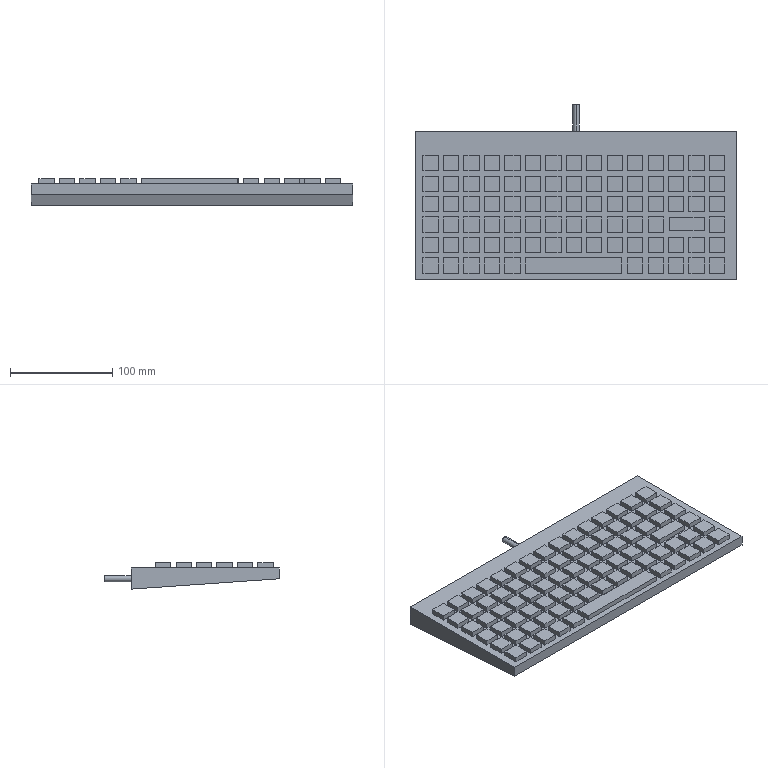Part | STEP file | Shuangfeiyankeyboard-FK112r | 1 solid | 434 faces | box 314 x 171 x 25.65 mm | volume 812761 mm3 | plane 432 | cylinder 2 | commonest cylinder face diameters 6 x2